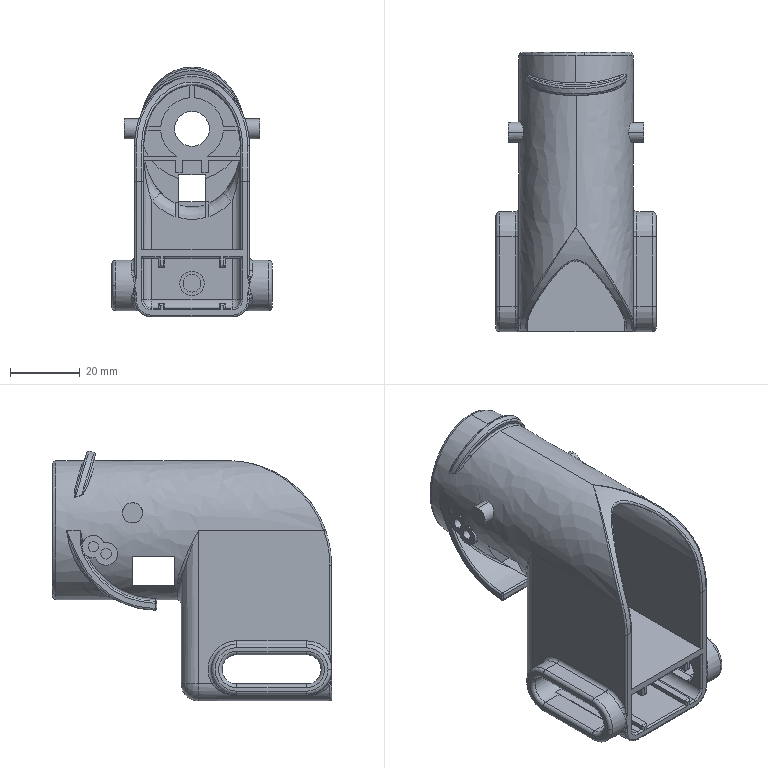Part | SolidWorks | features BaseBody 1 | 1 solid | 313 faces | box 46 x 80.21 x 71.833 mm | volume 45997 mm3 | cylinder 113 | plane 103 | spline 62 | torus 27 | sphere 8 | commonest cylinder face diameters 1 x33 2 x12 6.5 x12 5 x11 10 x9 3 x8